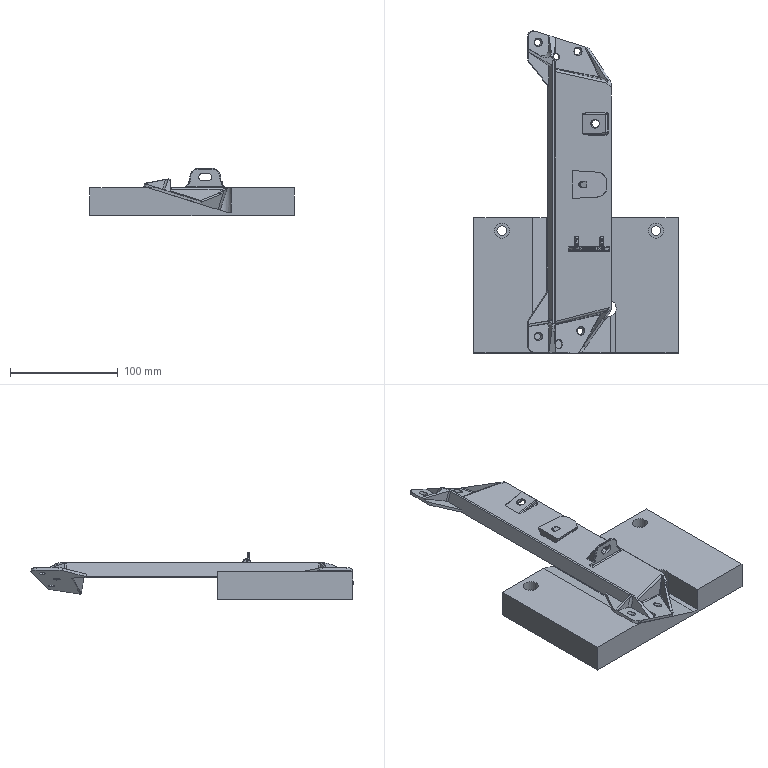NC program | NX | posted with a generic post | part box 190 x 299.709 x 43.804 mm
Whole program:
N10 G17 G21 G94 G90
(VARIABLE_AXIS_GUIDING_CURVES , TOOL : R3)
N12 T04 M6
N14 G54
N16 G17 G0 G90 X-7.631 Y8.378 S6800 M3
N18 G43 Z50.151 H4
N20 Z2.984
N22 G94 G1 Z-4.237 F2500.
N24 X-7.621 Y8.462 Z-4.713
N26 X-7.609 Y8.698 Z-5.403
N28 X-7.62 Y8.931 Z-6.093
N30 X-7.643 Y9.063 Z-6.56
N32 X-7.677 Y9.173 Z-7.032
N34 X-7.723 Y9.259 Z-7.508
N36 X-7.779 Y9.323 Z-7.987
N38 X-7.843 Y9.365 Z-8.467
N40 X-7.886 Y9.31 Z-8.612
N42 X-7.984 Y9.178 Z-8.937
N44 X-8.087 Y9.032 Z-9.254
N46 X-8.196 Y8.867 Z-9.56
N48 X-8.311 Y8.68 Z-9.85
N50 X-8.434 Y8.465 Z-10.116
N52 X-8.567 Y8.212 Z-10.341
N54 X-8.713 Y7.911 Z-10.477
N56 X-8.848 Y7.6 Z-10.386
N58 X-8.891 Y7.49 Z-10.051
N60 Z2.263
N62 G0 Z50.151
N64 X-29.481 Y-2.398
N66 Z-29.163
N68 G1 Z-36.911
N70 X-29.415 Y-2.296 Z-37.254
N72 X-29.208 Y-2.028 Z-37.384
N74 X-28.961 Y-1.762 Z-37.306
N76 X-28.718 Y-1.539 Z-37.133
N78 X-28.483 Y-1.351 Z-36.912
N80 X-28.255 Y-1.191 Z-36.663
N82 X-28.034 Y-1.054 Z-36.395
N84 X-27.819 Y-0.935 Z-36.114
N86 X-27.608 Y-0.831 Z-35.824
N88 X-27.459 Y-0.761 Z-35.612
N90 X-27.225 Y-0.626 Z-35.3
N92 X-27.009 Y-0.477 Z-35.032
N94 X-26.801 Y-0.315 Z-34.791
N96 X-26.678 Y-0.212 Z-34.657
N98 X-26.416 Y0.037 Z-34.385
N100 X-26.168 Y0.307 Z-34.149
N102 X-26.017 Y0.49 Z-34.015
N104 X-25.804 Y0.77 Z-33.838
N106 X-25.594 Y1.084 Z-33.678
N108 X-25.24 Y1.661 Z-33.444
N110 X-25.035 Y2.013 Z-33.305
N112 X-24.924 Y2.209 Z-33.221
N114 X-24.844 Y2.354 Z-33.14
N116 X-24.781 Y2.46 Z-33.049
N118 X-24.718 Y2.541 Z-32.933
N120 X-24.643 Y2.61 Z-32.78
N122 X-24.538 Y2.681 Z-32.574
N124 X-24.427 Y2.748 Z-32.363
N126 X-23.706 Y3.042 Z-31.309
N128 X-23.211 Y3.238 Z-30.591
N130 X-22.714 Y3.44 Z-29.876
N132 X-22.255 Y3.624 Z-29.213
N134 X-21.312 Y4.002 Z-27.85
N136 X-20.369 Y4.38 Z-26.487
N138 X-19.426 Y4.758 Z-25.124
N140 X-18.483 Y5.137 Z-23.761
N142 X-17.54 Y5.515 Z-22.398
N144 X-16.597 Y5.893 Z-21.035
N146 X-15.654 Y6.271 Z-19.672
N148 X-14.711 Y6.649 Z-18.309
N150 X-13.768 Y7.027 Z-16.946
N152 X-12.825 Y7.406 Z-15.583
N154 X-11.882 Y7.784 Z-14.22
N156 X-10.939 Y8.162 Z-12.857
N158 X-9.996 Y8.54 Z-11.494
N160 X-9.053 Y8.919 Z-10.131
N162 X-8.11 Y9.297 Z-8.768
N164 X-8.023 Y9.361 Z-8.579
N166 X-7.985 Y9.409 Z-8.452
N168 X-8.128 Y9.454 Z-8.437
N170 X-8.189 Y9.386 Z-8.62
N172 X-8.266 Y9.341 Z-8.761
N174 X-9.206 Y8.964 Z-10.118
N176 X-10.145 Y8.587 Z-11.475
N178 X-11.084 Y8.21 Z-12.832
N180 X-12.024 Y7.833 Z-14.189
N182 X-12.963 Y7.456 Z-15.546
N184 X-13.902 Y7.079 Z-16.903
N186 X-14.842 Y6.703 Z-18.26
N188 X-15.781 Y6.326 Z-19.617
N190 X-16.72 Y5.95 Z-20.974
N192 X-17.659 Y5.574 Z-22.331
N194 X-18.599 Y5.197 Z-23.689
N196 X-19.538 Y4.821 Z-25.046
N198 X-20.477 Y4.445 Z-26.403
N200 X-21.416 Y4.069 Z-27.761
N202 X-22.355 Y3.693 Z-29.118
N204 X-23.294 Y3.317 Z-30.476
N206 X-23.733 Y3.137 Z-31.11
N208 X-24.171 Y2.964 Z-31.747
N210 X-24.567 Y2.798 Z-32.334
N212 X-24.654 Y2.743 Z-32.503
N214 X-24.756 Y2.672 Z-32.71
N216 X-24.831 Y2.602 Z-32.864
N218 X-24.892 Y2.52 Z-32.981
N220 X-24.956 Y2.414 Z-33.072
N222 X-25.037 Y2.27 Z-33.153
N224 X-25.151 Y2.074 Z-33.236
N226 X-25.609 Y1.307 Z-33.539
N228 X-25.829 Y0.968 Z-33.693
N230 X-26.017 Y0.703 Z-33.846
N232 X-26.258 Y0.402 Z-34.054
N234 X-26.472 Y0.163 Z-34.256
N236 X-26.678 Y-0.042 Z-34.464
N238 X-26.806 Y-0.159 Z-34.598
N240 X-27.009 Y-0.325 Z-34.825
N242 X-27.255 Y-0.506 Z-35.119
N244 X-27.473 Y-0.642 Z-35.402
N246 X-27.725 Y-0.769 Z-35.752
N248 X-27.841 Y-0.706 Z-35.682
N250 X-27.67 Y-0.622 Z-35.442
N252 X-27.418 Y-0.473 Z-35.107
N254 X-27.229 Y-0.341 Z-34.876
N256 X-27.059 Y-0.21 Z-34.678
N258 X-26.839 Y-0.02 Z-34.44
N260 X-26.582 Y0.234 Z-34.178
N262 X-26.392 Y0.445 Z-33.999
N264 X-26.14 Y0.759 Z-33.781
N266 X-25.945 Y1.033 Z-33.622
N268 X-25.712 Y1.393 Z-33.458
N270 X-25.268 Y2.136 Z-33.166
N272 X-25.155 Y2.333 Z-33.082
N274 X-25.076 Y2.478 Z-33.001
N276 X-25.013 Y2.585 Z-32.909
N278 X-24.953 Y2.667 Z-32.793
N280 X-24.878 Y2.737 Z-32.638
N282 X-24.774 Y2.808 Z-32.432
N284 X-24.694 Y2.857 Z-32.28
N286 X-24.147 Y3.084 Z-31.471
N288 X-23.372 Y3.396 Z-30.348
N290 X-22.436 Y3.771 Z-28.996
N292 X-21.5 Y4.145 Z-27.643
N294 X-20.565 Y4.52 Z-26.291
N296 X-19.629 Y4.894 Z-24.939
N298 X-18.693 Y5.269 Z-23.587
N300 X-17.757 Y5.644 Z-22.234
N302 X-16.822 Y6.019 Z-20.882
N304 X-15.886 Y6.394 Z-19.53
N306 X-14.95 Y6.769 Z-18.178
N308 X-14.014 Y7.144 Z-16.826
N310 X-13.078 Y7.52 Z-15.474
N312 X-12.143 Y7.895 Z-14.122
N314 X-11.207 Y8.271 Z-12.771
N316 X-10.271 Y8.646 Z-11.419
N318 X-9.335 Y9.022 Z-10.067
N320 X-8.399 Y9.398 Z-8.715
N322 X-8.316 Y9.446 Z-8.562
N324 X-8.27 Y9.499 Z-8.422
N326 X-8.413 Y9.543 Z-8.407
N328 X-8.464 Y9.489 Z-8.554
N330 X-8.56 Y9.443 Z-8.709
N332 X-9.495 Y9.068 Z-10.06
N334 X-10.43 Y8.692 Z-11.41
N336 X-11.365 Y8.317 Z-12.761
N338 X-12.3 Y7.942 Z-14.112
N340 X-13.235 Y7.567 Z-15.463
N342 X-14.171 Y7.192 Z-16.814
N344 X-15.106 Y6.817 Z-18.165
N346 X-16.041 Y6.442 Z-19.515
N348 X-16.976 Y6.067 Z-20.866
N350 X-17.911 Y5.693 Z-22.217
N352 X-18.846 Y5.318 Z-23.568
N354 X-19.781 Y4.944 Z-24.92
N356 X-20.716 Y4.569 Z-26.271
N358 X-21.65 Y4.195 Z-27.622
N360 X-22.585 Y3.821 Z-28.973
N362 X-23.52 Y3.447 Z-30.325
N364 X-24.312 Y3.128 Z-31.471
N366 X-24.795 Y2.93 Z-32.179
N368 X-24.894 Y2.873 Z-32.36
N370 X-25. Y2.803 Z-32.565
N372 X-25.076 Y2.733 Z-32.719
N374 X-25.136 Y2.651 Z-32.836
N376 X-25.197 Y2.543 Z-32.928
N378 X-25.275 Y2.398 Z-33.01
N380 X-25.387 Y2.201 Z-33.094
N382 X-25.862 Y1.403 Z-33.409
N384 X-26.078 Y1.073 Z-33.564
N386 X-26.179 Y0.927 Z-33.645
N388 X-26.348 Y0.706 Z-33.787
N390 X-26.497 Y0.521 Z-33.918
N392 X-26.701 Y0.295 Z-34.11
N394 X-26.993 Y0.009 Z-34.408
N396 X-27.162 Y-0.135 Z-34.592
N398 X-27.34 Y-0.272 Z-34.799
N400 X-27.486 Y-0.378 Z-34.975
N402 X-27.67 Y-0.493 Z-35.214
N404 X-27.841 Y-0.588 Z-35.446
N406 X-27.958 Y-0.642 Z-35.612
N408 X-28.074 Y-0.578 Z-35.541
N410 X-27.865 Y-0.474 Z-35.248
N412 X-27.728 Y-0.396 Z-35.065
N414 X-27.509 Y-0.247 Z-34.791
N416 X-27.264 Y-0.06 Z-34.505
N418 X-27.064 Y0.115 Z-34.29
N420 X-26.767 Y0.413 Z-33.99
N422 X-26.538 Y0.679 Z-33.78
N424 X-26.279 Y1.014 Z-33.56
N426 X-26.02 Y1.403 Z-33.365
N428 X-25.509 Y2.256 Z-33.026
N430 X-25.505 Y2.265 Z-33.022
N432 X-25.418 Y2.469 Z-32.927
N434 X-25.345 Y2.616 Z-32.843
N436 X-25.276 Y2.721 Z-32.754
N438 X-25.203 Y2.799 Z-32.643
N440 X-25.118 Y2.866 Z-32.494
N442 X-25.01 Y2.936 Z-32.289
N444 X-24.933 Y2.985 Z-32.14
N446 X-24.476 Y3.172 Z-31.471
N448 X-24.051 Y3.34 Z-30.852
N450 X-23.625 Y3.515 Z-30.237
N452 X-22.677 Y3.894 Z-28.867
N454 X-21.729 Y4.273 Z-27.497
N456 X-20.781 Y4.653 Z-26.127
N458 X-19.834 Y5.032 Z-24.757
N460 X-18.886 Y5.412 Z-23.388
N462 X-17.938 Y5.792 Z-22.018
N464 X-16.99 Y6.172 Z-20.648
N466 X-16.042 Y6.552 Z-19.278
N468 X-15.094 Y6.932 Z-17.909
N470 X-14.146 Y7.312 Z-16.539
N472 X-13.198 Y7.693 Z-15.17
N474 X-12.249 Y8.073 Z-13.8
N476 X-11.301 Y8.454 Z-12.431
N478 X-10.353 Y8.834 Z-11.062
N480 X-9.479 Y9.186 Z-9.795
N482 X-8.605 Y9.539 Z-8.528
N484 X-8.555 Y9.588 Z-8.392
N486 X-8.697 Y9.633 Z-8.377
N488 X-8.741 Y9.592 Z-8.49
N490 X-9.678 Y9.216 Z-9.844
N492 X-10.615 Y8.84 Z-11.197
N494 X-11.552 Y8.464 Z-12.551
N496 X-12.489 Y8.088 Z-13.905
N498 X-13.426 Y7.712 Z-15.258
N500 X-14.363 Y7.336 Z-16.612
N502 X-15.3 Y6.96 Z-17.966
N504 X-16.237 Y6.585 Z-19.32
N506 X-17.174 Y6.209 Z-20.674
N508 X-18.11 Y5.834 Z-22.027
N510 X-19.047 Y5.458 Z-23.381
N512 X-19.984 Y5.083 Z-24.735
N514 X-20.921 Y4.708 Z-26.089
N516 X-21.858 Y4.333 Z-27.443
N518 X-22.794 Y3.957 Z-28.798
N520 X-23.731 Y3.582 Z-30.152
N522 X-24.172 Y3.402 Z-30.789
N524 X-24.612 Y3.227 Z-31.43
N526 X-25.06 Y3.044 Z-32.084
N528 X-25.131 Y3.002 Z-32.217
N530 X-25.243 Y2.933 Z-32.419
N532 X-25.331 Y2.867 Z-32.568
N534 X-25.403 Y2.788 Z-32.679
N536 X-25.471 Y2.683 Z-32.769
N538 X-25.542 Y2.535 Z-32.853
N540 X-25.627 Y2.33 Z-32.95
N542 X-25.641 Y2.295 Z-32.966
N544 X-26.124 Y1.486 Z-33.286
N546 X-26.402 Y1.07 Z-33.494
N548 X-26.655 Y0.741 Z-33.709
N550 X-26.848 Y0.514 Z-33.885
N552 X-27.009 Y0.346 Z-34.044
N554 X-27.177 Y0.182 Z-34.216
N556 X-27.385 Y-0.001 Z-34.44
N558 X-27.67 Y-0.217 Z-34.774
N560 X-27.845 Y-0.333 Z-34.994
N562 X-28.095 Y-0.471 Z-35.336
N564 X-28.19 Y-0.516 Z-35.47
N566 X-28.306 Y-0.452 Z-35.399
N568 X-28.078 Y-0.337 Z-35.08
N570 X-27.857 Y-0.201 Z-34.791
N572 X-27.613 Y-0.025 Z-34.497
N574 X-27.42 Y0.131 Z-34.279
N576 X-27.107 Y0.429 Z-33.953
N578 X-26.933 Y0.615 Z-33.785
N580 X-26.737 Y0.848 Z-33.609
N582 X-26.536 Y1.113 Z-33.437
N584 X-26.342 Y1.396 Z-33.287
N586 X-26.23 Y1.567 Z-33.208
N588 X-25.786 Y2.308 Z-32.915
N590 X-25.75 Y2.396 Z-32.876
N592 X-25.662 Y2.599 Z-32.781
N594 X-25.588 Y2.746 Z-32.698
N596 X-25.518 Y2.851 Z-32.609
N598 X-25.444 Y2.929 Z-32.499
N600 X-25.357 Y2.995 Z-32.35
N602 X-25.247 Y3.065 Z-32.146
N604 X-25.201 Y3.094 Z-32.057
N606 X-24.694 Y3.305 Z-31.309
N608 X-23.896 Y3.626 Z-30.152
N610 X-22.957 Y4.002 Z-28.794
N612 X-22.019 Y4.378 Z-27.437
N614 X-21.08 Y4.753 Z-26.08
N616 X-20.141 Y5.129 Z-24.723
N618 X-19.202 Y5.505 Z-23.366
N620 X-18.263 Y5.882 Z-22.009
N622 X-17.324 Y6.258 Z-20.652
N624 X-16.385 Y6.634 Z-19.295
N626 X-15.446 Y7.011 Z-17.938
N628 X-14.507 Y7.387 Z-16.582
N630 X-13.568 Y7.764 Z-15.225
N632 X-12.629 Y8.141 Z-13.868
N634 X-11.69 Y8.518 Z-12.512
N636 X-10.751 Y8.895 Z-11.155
N638 X-9.812 Y9.272 Z-9.799
N640 X-8.873 Y9.649 Z-8.442
N642 X-8.84 Y9.677 Z-8.362
N644 X-8.982 Y9.722 Z-8.347
N646 X-9.033 Y9.693 Z-8.438
N648 X-9.094 Y9.669 Z-8.526
N650 X-10.023 Y9.296 Z-9.868
N652 X-10.952 Y8.923 Z-11.21
N654 X-11.881 Y8.55 Z-12.552
N656 X-12.81 Y8.178 Z-13.894
N658 X-13.739 Y7.805 Z-15.236
N660 X-14.668 Y7.432 Z-16.578
N662 X-15.597 Y7.06 Z-17.92
N664 X-16.526 Y6.688 Z-19.262
N666 X-17.455 Y6.315 Z-20.605
N668 X-18.384 Y5.943 Z-21.947
N670 X-19.313 Y5.571 Z-23.289
N672 X-20.242 Y5.199 Z-24.632
N674 X-21.171 Y4.827 Z-25.974
N676 X-22.1 Y4.455 Z-27.317
N678 X-23.029 Y4.083 Z-28.659
N680 X-23.958 Y3.712 Z-30.002
N682 X-24.741 Y3.396 Z-31.137
N684 X-25.313 Y3.162 Z-31.973
N686 X-25.365 Y3.129 Z-32.075
N688 X-25.474 Y3.059 Z-32.279
N690 X-25.562 Y2.993 Z-32.427
N692 X-25.638 Y2.915 Z-32.537
N694 X-25.709 Y2.811 Z-32.625
N696 X-25.784 Y2.664 Z-32.708
N698 X-25.871 Y2.461 Z-32.803
N700 X-25.912 Y2.357 Z-32.85
N702 X-26.348 Y1.63 Z-33.138
N704 X-26.558 Y1.311 Z-33.29
N706 X-26.757 Y1.034 Z-33.455
N708 X-27.009 Y0.724 Z-33.677
N710 X-27.202 Y0.513 Z-33.861
N712 X-27.521 Y0.208 Z-34.192
N714 X-27.741 Y0.03 Z-34.44
N716 X-28.013 Y-0.164 Z-34.77
N718 X-28.219 Y-0.287 Z-35.043
N720 X-28.422 Y-0.389 Z-35.329
N722 X-28.538 Y-0.326 Z-35.258
N724 X-28.258 Y-0.179 Z-34.868
N726 X-28.069 Y-0.059 Z-34.626
N728 X-27.779 Y0.154 Z-34.278
N730 X-27.588 Y0.316 Z-34.07
N732 X-27.308 Y0.587 Z-33.78
N734 X-27.112 Y0.803 Z-33.594
N736 X-26.828 Y1.157 Z-33.346
N738 X-26.649 Y1.414 Z-33.199
N740 X-26.404 Y1.79 Z-33.028
N742 X-26.038 Y2.406 Z-32.785
N744 X-25.991 Y2.525 Z-32.731
N746 X-25.904 Y2.729 Z-32.636
N748 X-25.828 Y2.875 Z-32.553
N750 X-25.754 Y2.978 Z-32.466
N752 X-25.677 Y3.055 Z-32.357
N754 X-25.588 Y3.121 Z-32.209
N756 X-25.482 Y3.193 Z-32.004
N758 X-25.44 Y3.222 Z-31.917
N760 X-24.694 Y3.526 Z-30.828
N762 X-24.234 Y3.708 Z-30.161
N764 X-23.773 Y3.896 Z-29.496
N766 X-23.592 Y3.968 Z-29.235
N768 X-22.628 Y4.354 Z-27.842
N770 X-21.663 Y4.741 Z-26.448
N772 X-20.699 Y5.127 Z-25.054
N774 X-19.734 Y5.513 Z-23.661
N776 X-18.77 Y5.9 Z-22.267
N778 X-17.805 Y6.286 Z-20.873
N780 X-16.841 Y6.673 Z-19.48
N782 X-15.876 Y7.06 Z-18.086
N784 X-14.912 Y7.446 Z-16.693
N786 X-13.947 Y7.833 Z-15.299
N788 X-12.983 Y8.22 Z-13.906
N790 X-12.018 Y8.606 Z-12.512
N792 X-11.054 Y8.993 Z-11.119
N794 X-10.089 Y9.38 Z-9.725
N796 X-9.125 Y9.767 Z-8.332
N798 X-9.279 Y9.815 Z-8.316
N800 X-10.213 Y9.44 Z-9.666
N802 X-11.148 Y9.065 Z-11.015
N804 X-12.083 Y8.69 Z-12.365
N806 X-13.017 Y8.315 Z-13.715
N808 X-13.952 Y7.94 Z-15.065
N810 X-14.886 Y7.565 Z-16.415
N812 X-15.821 Y7.19 Z-17.765
N814 X-16.755 Y6.816 Z-19.116
N816 X-17.69 Y6.441 Z-20.466
N818 X-18.624 Y6.067 Z-21.816
N820 X-19.559 Y5.693 Z-23.166
N822 X-20.493 Y5.318 Z-24.517
N824 X-21.427 Y4.944 Z-25.867
N826 X-22.362 Y4.57 Z-27.217
N828 X-23.296 Y4.196 Z-28.568
N830 X-24.23 Y3.822 Z-29.918
N832 X-25.054 Y3.49 Z-31.112
N834 X-25.54 Y3.291 Z-31.824
N836 X-25.6 Y3.257 Z-31.933
N838 X-25.713 Y3.189 Z-32.135
N840 X-25.804 Y3.123 Z-32.283
N842 X-25.881 Y3.046 Z-32.392
N844 X-25.953 Y2.941 Z-32.479
N846 X-26.027 Y2.794 Z-32.563
N848 X-26.112 Y2.59 Z-32.658
N850 X-26.17 Y2.445 Z-32.724
N852 X-26.607 Y1.717 Z-33.013
N854 X-26.827 Y1.388 Z-33.176
N856 X-27.041 Y1.097 Z-33.355
N858 X-27.227 Y0.869 Z-33.522
N860 X-27.441 Y0.634 Z-33.726
N862 X-27.77 Y0.321 Z-34.068
N864 X-27.906 Y0.209 Z-34.22
N866 X-28.199 Y-0.006 Z-34.571
N868 X-28.355 Y-0.105 Z-34.77
N870 X-28.655 Y-0.262 Z-35.187
N872 X-28.771 Y-0.199 Z-35.116
N874 X-28.524 Y-0.072 Z-34.77
N876 X-28.294 Y0.072 Z-34.473
N878 X-28.001 Y0.289 Z-34.125
N880 X-27.782 Y0.48 Z-33.887
N882 X-27.563 Y0.692 Z-33.66
N884 X-27.343 Y0.934 Z-33.451
N886 X-27.145 Y1.176 Z-33.274
N888 X-26.991 Y1.383 Z-33.143
N890 X-26.736 Y1.763 Z-32.95
N892 X-26.302 Y2.484 Z-32.663
N894 X-26.233 Y2.655 Z-32.586
N896 X-26.147 Y2.859 Z-32.491
N898 X-26.071 Y3.005 Z-32.408
N900 X-25.998 Y3.109 Z-32.321
N902 X-25.921 Y3.187 Z-32.212
N904 X-25.831 Y3.253 Z-32.064
N906 X-25.721 Y3.322 Z-31.861
N908 X-25.703 Y3.333 Z-31.827
N910 X-25.135 Y3.568 Z-30.99
N912 X-24.321 Y3.896 Z-29.81
N914 X-23.39 Y4.268 Z-28.465
N916 X-22.46 Y4.641 Z-27.121
N918 X-21.529 Y5.013 Z-25.776
N920 X-20.599 Y5.386 Z-24.431
N922 X-19.669 Y5.759 Z-23.087
N924 X-18.738 Y6.131 Z-21.742
N926 X-17.808 Y6.504 Z-20.398
N928 X-16.877 Y6.877 Z-19.053
N930 X-15.947 Y7.25 Z-17.709
N932 X-15.016 Y7.623 Z-16.365
N934 X-14.086 Y7.996 Z-15.02
N936 X-13.155 Y8.37 Z-13.676
N938 X-12.225 Y8.743 Z-12.332
N940 X-11.294 Y9.116 Z-10.988
N942 X-10.363 Y9.49 Z-9.644
N944 X-9.433 Y9.863 Z-8.3
N946 X-9.587 Y9.912 Z-8.283
N948 X-10.544 Y9.528 Z-9.667
N950 X-11.502 Y9.143 Z-11.05
N952 X-12.46 Y8.759 Z-12.434
N954 X-13.417 Y8.376 Z-13.818
N956 X-14.375 Y7.992 Z-15.201
N958 X-15.333 Y7.608 Z-16.585
N960 X-16.29 Y7.224 Z-17.968
N962 X-17.248 Y6.84 Z-19.352
N964 X-18.206 Y6.456 Z-20.736
N966 X-19.163 Y6.072 Z-22.119
N968 X-20.121 Y5.689 Z-23.503
N970 X-21.078 Y5.305 Z-24.887
N972 X-22.036 Y4.921 Z-26.271
N974 X-22.994 Y4.538 Z-27.654
N976 X-23.951 Y4.154 Z-29.038
N978 X-24.253 Y4.033 Z-29.474
N980 X-24.695 Y3.854 Z-30.11
N982 X-25.135 Y3.679 Z-30.749
N984 X-25.805 Y3.405 Z-31.73
N986 X-25.837 Y3.385 Z-31.791
N988 X-25.947 Y3.316 Z-31.994
N990 X-26.037 Y3.25 Z-32.141
N992 X-26.115 Y3.173 Z-32.25
N994 X-26.188 Y3.069 Z-32.337
N996 X-26.265 Y2.923 Z-32.419
N998 X-26.353 Y2.72 Z-32.514
N1000 X-26.433 Y2.523 Z-32.602
N1002 X-26.855 Y1.823 Z-32.881
N1004 X-27.084 Y1.482 Z-33.052
N1006 X-27.249 Y1.255 Z-33.192
N1008 X-27.481 Y0.974 Z-33.399
N1010 X-27.69 Y0.745 Z-33.6
N1012 X-27.899 Y0.544 Z-33.816
N1014 X-28.125 Y0.347 Z-34.063
N1016 X-28.372 Y0.162 Z-34.355
N1018 X-28.551 Y0.044 Z-34.582
N1020 X-28.775 Y-0.08 Z-34.885
N1022 X-28.887 Y-0.134 Z-35.046
N1024 X-29.003 Y-0.07 Z-34.975
N1026 X-28.812 Y0.024 Z-34.704
N1028 X-28.598 Y0.151 Z-34.422
N1030 X-28.363 Y0.316 Z-34.134
N1032 X-28.143 Y0.492 Z-33.882
N1034 X-27.93 Y0.686 Z-33.656
N1036 X-27.703 Y0.917 Z-33.428
N1038 X-27.479 Y1.178 Z-33.221
N1040 X-27.319 Y1.381 Z-33.08
N1042 X-27.18 Y1.576 Z-32.965
N1044 X-26.974 Y1.883 Z-32.811
N1046 X-26.565 Y2.562 Z-32.541
N1048 X-26.475 Y2.785 Z-32.441
N1050 X-26.388 Y2.988 Z-32.346
N1052 X-26.311 Y3.135 Z-32.264
N1054 X-26.238 Y3.239 Z-32.177
N1056 X-26.16 Y3.316 Z-32.069
N1058 X-26.069 Y3.381 Z-31.921
N1060 X-25.957 Y3.45 Z-31.719
N1062 X-25.942 Y3.459 Z-31.691
N1064 X-25.493 Y3.644 Z-31.031
N1066 X-25.039 Y3.824 Z-30.371
N1068 X-24.585 Y4.01 Z-29.714
N1070 X-23.657 Y4.382 Z-28.373
N1072 X-22.729 Y4.753 Z-27.033
N1074 X-21.802 Y5.124 Z-25.692
N1076 X-20.874 Y5.496 Z-24.351
N1078 X-19.946 Y5.867 Z-23.011
N1080 X-19.019 Y6.239 Z-21.67
N1082 X-18.091 Y6.61 Z-20.33
N1084 X-17.163 Y6.982 Z-18.989
N1086 X-16.236 Y7.354 Z-17.649
N1088 X-15.308 Y7.726 Z-16.308
N1090 X-14.38 Y8.098 Z-14.968
N1092 X-13.452 Y8.47 Z-13.628
N1094 X-12.524 Y8.843 Z-12.288
N1096 X-11.596 Y9.215 Z-10.947
N1098 X-10.669 Y9.587 Z-9.607
N1100 X-9.741 Y9.96 Z-8.267
N1102 X-9.894 Y10.008 Z-8.251
N1104 X-10.872 Y9.616 Z-9.663
N1106 X-11.85 Y9.224 Z-11.075
N1108 X-12.827 Y8.832 Z-12.487
N1110 X-13.805 Y8.44 Z-13.899
N1112 X-14.782 Y8.048 Z-15.311
N1114 X-15.76 Y7.656 Z-16.723
N1116 X-16.737 Y7.264 Z-18.136
N1118 X-17.715 Y6.872 Z-19.548
N1120 X-18.692 Y6.48 Z-20.96
N1122 X-19.67 Y6.089 Z-22.372
N1124 X-20.647 Y5.697 Z-23.785
N1126 X-21.624 Y5.306 Z-25.197
N1128 X-22.602 Y4.914 Z-26.61
N1130 X-23.579 Y4.523 Z-28.022
N1132 X-24.557 Y4.132 Z-29.435
N1134 X-25.357 Y3.811 Z-30.592
N1136 X-26.069 Y3.518 Z-31.637
N1138 X-26.075 Y3.514 Z-31.647
N1140 X-26.186 Y3.445 Z-31.85
N1142 X-26.278 Y3.38 Z-31.997
N1144 X-26.356 Y3.303 Z-32.106
N1146 X-26.43 Y3.199 Z-32.192
N1148 X-26.507 Y3.053 Z-32.274
N1150 X-26.596 Y2.849 Z-32.368
N1152 X-26.697 Y2.601 Z-32.48
N1154 X-27.061 Y1.995 Z-32.72
N1156 X-27.266 Y1.684 Z-32.87
N1158 X-27.418 Y1.467 Z-32.995
N1160 X-27.608 Y1.227 Z-33.16
N1162 X-27.823 Y0.978 Z-33.36
N1164 X-28.067 Y0.731 Z-33.606
N1166 X-28.265 Y0.549 Z-33.818
N1168 X-28.492 Y0.37 Z-34.077
N1170 X-28.732 Y0.203 Z-34.373
N1172 X-28.983 Y0.058 Z-34.709
N1174 X-29.119 Y-0.007 Z-34.903
N1176 X-29.235 Y0.056 Z-34.832
N1178 X-29.078 Y0.132 Z-34.608
N1180 X-28.831 Y0.278 Z-34.279
N1182 X-28.643 Y0.408 Z-34.047
N1184 X-28.411 Y0.589 Z-33.781
N1186 X-28.17 Y0.805 Z-33.52
N1188 X-27.94 Y1.041 Z-33.29
N1190 X-27.727 Y1.287 Z-33.091
N1192 X-27.521 Y1.551 Z-32.912
N1194 X-27.308 Y1.86 Z-32.742
N1196 X-27.213 Y2.002 Z-32.674
N1198 X-26.833 Y2.634 Z-32.421
N1200 X-26.72 Y2.918 Z-32.293
N1202 X-26.636 Y3.123 Z-32.196
N1204 X-26.565 Y3.272 Z-32.111
N1206 X-26.496 Y3.379 Z-32.021
N1208 X-26.418 Y3.456 Z-31.912
N1210 X-26.319 Y3.518 Z-31.768
N1212 X-26.188 Y3.578 Z-31.574
N1214 X-25.627 Y3.811 Z-30.747
N1216 X-24.797 Y4.145 Z-29.543
N1218 X-23.814 Y4.539 Z-28.122
N1220 X-22.831 Y4.932 Z-26.701
N1222 X-21.847 Y5.326 Z-25.28
N1224 X-20.864 Y5.72 Z-23.86
N1226 X-19.881 Y6.113 Z-22.439
N1228 X-18.898 Y6.507 Z-21.018
N1230 X-17.915 Y6.901 Z-19.598
N1232 X-16.932 Y7.295 Z-18.177
N1234 X-15.948 Y7.69 Z-16.757
N1236 X-14.965 Y8.084 Z-15.336
N1238 X-13.982 Y8.478 Z-13.916
N1240 X-12.999 Y8.873 Z-12.496
N1242 X-12.015 Y9.267 Z-11.075
N1244 X-11.032 Y9.662 Z-9.655
N1246 X-10.049 Y10.056 Z-8.235
N1248 X-10.203 Y10.103 Z-8.218
N1250 X-11.191 Y9.706 Z-9.645
N1252 X-12.18 Y9.31 Z-11.073
N1254 X-13.168 Y8.913 Z-12.5
N1256 X-14.156 Y8.517 Z-13.928
N1258 X-15.144 Y8.121 Z-15.355
N1260 X-16.132 Y7.725 Z-16.783
N1262 X-17.121 Y7.329 Z-18.211
N1264 X-18.109 Y6.933 Z-19.638
N1266 X-19.097 Y6.537 Z-21.066
N1268 X-20.085 Y6.141 Z-22.494
N1270 X-21.073 Y5.745 Z-23.922
N1272 X-22.061 Y5.35 Z-25.35
N1274 X-23.049 Y4.954 Z-26.778
N1276 X-24.037 Y4.559 Z-28.206
N1278 X-25.025 Y4.164 Z-29.634
N1280 X-25.481 Y3.977 Z-30.293
N1282 X-25.935 Y3.796 Z-30.956
N1284 X-26.307 Y3.641 Z-31.507
N1286 X-26.439 Y3.581 Z-31.701
N1288 X-26.539 Y3.519 Z-31.844
N1290 X-26.618 Y3.442 Z-31.952
N1292 X-26.687 Y3.335 Z-32.041
N1294 X-26.758 Y3.186 Z-32.126
N1296 X-26.842 Y2.98 Z-32.222
N1298 X-26.961 Y2.679 Z-32.357
N1300 X-27.34 Y2.051 Z-32.61
N1302 X-27.554 Y1.733 Z-32.77
N1304 X-27.8 Y1.403 Z-32.98
N1306 X-28.001 Y1.165 Z-33.166
N1308 X-28.179 Y0.975 Z-33.341
N1310 X-28.396 Y0.766 Z-33.565
N1312 X-28.662 Y0.544 Z-33.862
N1314 X-28.789 Y0.448 Z-34.012
N1316 X-29. Y0.309 Z-34.278
N1318 X-29.19 Y0.198 Z-34.531
N1320 X-29.351 Y0.119 Z-34.76
N1322 X-29.467 Y0.183 Z-34.689
N1324 X-29.259 Y0.288 Z-34.396
N1326 X-29. Y0.446 Z-34.057
N1328 X-28.851 Y0.55 Z-33.873
N1330 X-28.646 Y0.711 Z-33.638
N1332 X-28.466 Y0.868 Z-33.442
N1334 X-28.199 Y1.136 Z-33.169
N1336 X-27.992 Y1.373 Z-32.975
N1338 X-27.873 Y1.518 Z-32.869
N1340 X-27.662 Y1.808 Z-32.692
N1342 X-27.451 Y2.127 Z-32.534
N1344 X-27.103 Y2.703 Z-32.305
N1346 X-26.979 Y3.01 Z-32.166
N1348 X-26.961 Y3.043 Z-32.152
N1350 X-26.858 Y3.244 Z-32.064
N1352 X-26.781 Y3.392 Z-31.982
N1354 X-26.715 Y3.499 Z-31.892
N1356 X-26.645 Y3.579 Z-31.78
N1358 X-26.554 Y3.643 Z-31.633
N1360 X-26.425 Y3.704 Z-31.438
N1362 X-26.017 Y3.874 Z-30.835
N1364 X-25.992 Y3.884 Z-30.799
N1366 X-25.523 Y4.07 Z-30.116
N1368 X-25.053 Y4.263 Z-29.437
N1370 X-24.08 Y4.653 Z-28.03
N1372 X-23.106 Y5.043 Z-26.622
N1374 X-22.132 Y5.432 Z-25.215
N1376 X-21.158 Y5.822 Z-23.808
N1378 X-20.185 Y6.212 Z-22.401
N1380 X-19.211 Y6.603 Z-20.993
N1382 X-18.237 Y6.993 Z-19.586
N1384 X-17.263 Y7.383 Z-18.179
N1386 X-16.289 Y7.773 Z-16.772
N1388 X-15.315 Y8.164 Z-15.365
N1390 X-14.342 Y8.554 Z-13.959
N1392 X-13.368 Y8.945 Z-12.552
N1394 X-12.394 Y9.336 Z-11.145
N1396 X-11.42 Y9.727 Z-9.738
N1398 X-10.446 Y10.118 Z-8.331
N1400 X-10.347 Y10.152 Z-8.204
N1402 X-10.139 Y10.053 Z-7.782
N1404 X-9.944 Y9.935 Z-7.358
N1406 X-9.767 Y9.796 Z-6.934
N1408 X-9.608 Y9.638 Z-6.508
N1410 X-9.472 Y9.461 Z-6.082
N1412 X-9.361 Y9.27 Z-5.655
N1414 X-9.28 Y9.074 Z-5.224
N1416 X-9.232 Y8.894 Z-4.781
N1418 X-9.219 Y8.8 Z-4.312
N1420 Z2.534
N1422 G0 Z50.151
N1424 M5
N1426 M2